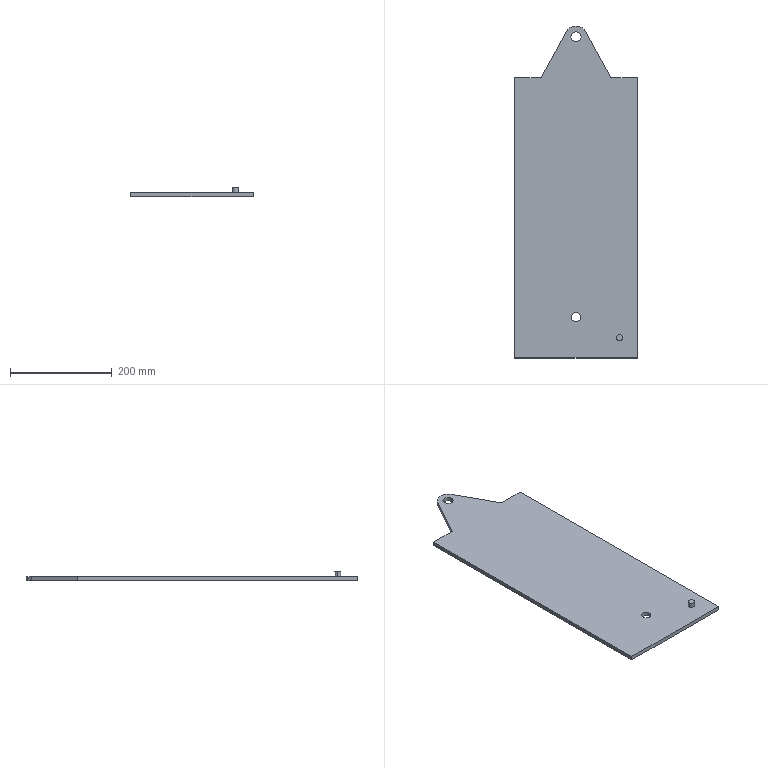Part | SolidWorks | features Extrusion 1, ICE 1 | 1 solid | 17 faces | box 240 x 651.329 x 18 mm | volume 1117831 mm3 | plane 10 | cylinder 7 | commonest cylinder face diameters 12 x2 18 x2 20 x2 42.659 x1
STEP:
#1=CARTESIAN_POINT('',(91.,40.,18.));
#2=VERTEX_POINT('',#1);
#3=CARTESIAN_POINT('',(79.,40.,18.));
#4=VERTEX_POINT('',#3);
#5=CARTESIAN_POINT('',(85.,40.,18.));
#6=DIRECTION('',(0.,0.,1.));
#7=DIRECTION('',(1.,0.,0.));
#8=AXIS2_PLACEMENT_3D('',#5,#6,#7);
#9=CIRCLE('',#8,6.);
#10=EDGE_CURVE('',#2,#4,#9,.T.);
#11=ORIENTED_EDGE('',*,*,#10,.F.);
#12=CARTESIAN_POINT('',(91.,40.,8.));
#13=VERTEX_POINT('',#12);
#14=CARTESIAN_POINT('',(91.,40.,18.));
#15=DIRECTION('',(0.,0.,-1.));
#16=VECTOR('',#15,1000.);
#17=LINE('',#14,#16);
#18=EDGE_CURVE('',#2,#13,#17,.T.);
#19=ORIENTED_EDGE('',*,*,#18,.T.);
#20=CARTESIAN_POINT('',(79.,40.,8.));
#21=VERTEX_POINT('',#20);
#22=CARTESIAN_POINT('',(85.,40.,8.));
#23=DIRECTION('',(0.,0.,1.));
#24=DIRECTION('',(1.,0.,0.));
#25=AXIS2_PLACEMENT_3D('',#22,#23,#24);
#26=CIRCLE('',#25,6.);
#27=EDGE_CURVE('',#13,#21,#26,.T.);
#28=ORIENTED_EDGE('',*,*,#27,.T.);
#29=CARTESIAN_POINT('',(79.,40.,18.));
#30=DIRECTION('',(0.,0.,-1.));
#31=VECTOR('',#30,1000.);
#32=LINE('',#29,#31);
#33=EDGE_CURVE('',#4,#21,#32,.T.);
#34=ORIENTED_EDGE('',*,*,#33,.F.);
#35=EDGE_LOOP('',(#11,#19,#28,#34));
#36=FACE_OUTER_BOUND('',#35,.T.);
#37=CARTESIAN_POINT('',(85.,40.,18.));
#38=DIRECTION('',(0.,0.,-1.));
#39=DIRECTION('',(-1.,0.,0.));
#40=AXIS2_PLACEMENT_3D('',#37,#38,#39);
#41=CYLINDRICAL_SURFACE('',#40,6.);
#42=ADVANCED_FACE('',(#36),#41,.T.);
#43=CARTESIAN_POINT('',(-9.,80.,8.));
#44=VERTEX_POINT('',#43);
#45=CARTESIAN_POINT('',(9.,80.,8.));
#46=VERTEX_POINT('',#45);
#47=CARTESIAN_POINT('',(0.,80.,8.));
#48=DIRECTION('',(0.,0.,1.));
#49=DIRECTION('',(1.,0.,0.));
#50=AXIS2_PLACEMENT_3D('',#47,#48,#49);
#51=CIRCLE('',#50,9.);
#52=EDGE_CURVE('',#44,#46,#51,.T.);
#53=ORIENTED_EDGE('',*,*,#52,.T.);
#54=CARTESIAN_POINT('',(9.,80.,0.));
#55=VERTEX_POINT('',#54);
#56=CARTESIAN_POINT('',(9.,80.,8.));
#57=DIRECTION('',(0.,0.,-1.));
#58=VECTOR('',#57,1000.);
#59=LINE('',#56,#58);
#60=EDGE_CURVE('',#46,#55,#59,.T.);
#61=ORIENTED_EDGE('',*,*,#60,.T.);
#62=CARTESIAN_POINT('',(-9.,80.,0.));
#63=VERTEX_POINT('',#62);
#64=CARTESIAN_POINT('',(0.,80.,0.));
#65=DIRECTION('',(0.,0.,1.));
#66=DIRECTION('',(1.,0.,0.));
#67=AXIS2_PLACEMENT_3D('',#64,#65,#66);
#68=CIRCLE('',#67,9.);
#69=EDGE_CURVE('',#63,#55,#68,.T.);
#70=ORIENTED_EDGE('',*,*,#69,.F.);
#71=CARTESIAN_POINT('',(-9.,80.,8.));
#72=DIRECTION('',(0.,0.,-1.));
#73=VECTOR('',#72,1000.);
#74=LINE('',#71,#73);
#75=EDGE_CURVE('',#44,#63,#74,.T.);
#76=ORIENTED_EDGE('',*,*,#75,.F.);
#77=EDGE_LOOP('',(#53,#61,#70,#76));
#78=FACE_OUTER_BOUND('',#77,.T.);
#79=CARTESIAN_POINT('',(0.,80.,8.));
#80=DIRECTION('',(0.,0.,-1.));
#81=DIRECTION('',(-1.,0.,0.));
#82=AXIS2_PLACEMENT_3D('',#79,#80,#81);
#83=CYLINDRICAL_SURFACE('',#82,9.);
#84=ADVANCED_FACE('',(#78),#83,.F.);
#85=CARTESIAN_POINT('',(-10.,630.,8.));
#86=VERTEX_POINT('',#85);
#87=CARTESIAN_POINT('',(10.,630.,8.));
#88=VERTEX_POINT('',#87);
#89=CARTESIAN_POINT('',(0.,630.,8.));
#90=DIRECTION('',(0.,0.,1.));
#91=DIRECTION('',(1.,0.,0.));
#92=AXIS2_PLACEMENT_3D('',#89,#90,#91);
#93=CIRCLE('',#92,10.);
#94=EDGE_CURVE('',#86,#88,#93,.T.);
#95=ORIENTED_EDGE('',*,*,#94,.T.);
#96=CARTESIAN_POINT('',(10.,630.,0.));
#97=VERTEX_POINT('',#96);
#98=CARTESIAN_POINT('',(10.,630.,8.));
#99=DIRECTION('',(0.,0.,-1.));
#100=VECTOR('',#99,1000.);
#101=LINE('',#98,#100);
#102=EDGE_CURVE('',#88,#97,#101,.T.);
#103=ORIENTED_EDGE('',*,*,#102,.T.);
#104=CARTESIAN_POINT('',(-10.,630.,0.));
#105=VERTEX_POINT('',#104);
#106=CARTESIAN_POINT('',(0.,630.,0.));
#107=DIRECTION('',(0.,0.,1.));
#108=DIRECTION('',(1.,0.,0.));
#109=AXIS2_PLACEMENT_3D('',#106,#107,#108);
#110=CIRCLE('',#109,10.);
#111=EDGE_CURVE('',#105,#97,#110,.T.);
#112=ORIENTED_EDGE('',*,*,#111,.F.);
#113=CARTESIAN_POINT('',(-10.,630.,8.));
#114=DIRECTION('',(0.,0.,-1.));
#115=VECTOR('',#114,1000.);
#116=LINE('',#113,#115);
#117=EDGE_CURVE('',#86,#105,#116,.T.);
#118=ORIENTED_EDGE('',*,*,#117,.F.);
#119=EDGE_LOOP('',(#95,#103,#112,#118));
#120=FACE_OUTER_BOUND('',#119,.T.);
#121=CARTESIAN_POINT('',(0.,630.,8.));
#122=DIRECTION('',(0.,0.,-1.));
#123=DIRECTION('',(-1.,0.,0.));
#124=AXIS2_PLACEMENT_3D('',#121,#122,#123);
#125=CYLINDRICAL_SURFACE('',#124,10.);
#126=ADVANCED_FACE('',(#120),#125,.F.);
#127=CARTESIAN_POINT('',(85.,40.,8.));
#128=DIRECTION('',(0.,0.,1.));
#129=DIRECTION('',(1.,0.,0.));
#130=AXIS2_PLACEMENT_3D('',#127,#128,#129);
#131=CIRCLE('',#130,6.);
#132=EDGE_CURVE('',#21,#13,#131,.T.);
#133=ORIENTED_EDGE('',*,*,#132,.F.);
#134=ORIENTED_EDGE('',*,*,#27,.F.);
#135=EDGE_LOOP('',(#133,#134));
#136=FACE_BOUND('',#135,.T.);
#137=ORIENTED_EDGE('',*,*,#94,.F.);
#138=CARTESIAN_POINT('',(0.,630.,8.));
#139=DIRECTION('',(0.,0.,1.));
#140=DIRECTION('',(1.,0.,0.));
#141=AXIS2_PLACEMENT_3D('',#138,#139,#140);
#142=CIRCLE('',#141,10.);
#143=EDGE_CURVE('',#88,#86,#142,.T.);
#144=ORIENTED_EDGE('',*,*,#143,.F.);
#145=EDGE_LOOP('',(#137,#144));
#146=FACE_BOUND('',#145,.T.);
#147=CARTESIAN_POINT('',(-120.,550.,8.));
#148=VERTEX_POINT('',#147);
#149=CARTESIAN_POINT('',(-120.,0.,8.));
#150=VERTEX_POINT('',#149);
#151=CARTESIAN_POINT('',(-120.,0.,8.));
#152=DIRECTION('',(0.,-1.,0.));
#153=VECTOR('',#152,1000.);
#154=LINE('',#151,#153);
#155=EDGE_CURVE('',#148,#150,#154,.T.);
#156=ORIENTED_EDGE('',*,*,#155,.T.);
#157=CARTESIAN_POINT('',(120.,0.,8.));
#158=VERTEX_POINT('',#157);
#159=CARTESIAN_POINT('',(120.,0.,8.));
#160=DIRECTION('',(1.,0.,0.));
#161=VECTOR('',#160,1000.);
#162=LINE('',#159,#161);
#163=EDGE_CURVE('',#150,#158,#162,.T.);
#164=ORIENTED_EDGE('',*,*,#163,.T.);
#165=CARTESIAN_POINT('',(120.,550.,8.));
#166=VERTEX_POINT('',#165);
#167=CARTESIAN_POINT('',(120.,550.,8.));
#168=DIRECTION('',(0.,1.,0.));
#169=VECTOR('',#168,1000.);
#170=LINE('',#167,#169);
#171=EDGE_CURVE('',#158,#166,#170,.T.);
#172=ORIENTED_EDGE('',*,*,#171,.T.);
#173=CARTESIAN_POINT('',(68.4,550.,8.));
#174=VERTEX_POINT('',#173);
#175=CARTESIAN_POINT('',(68.4,550.,8.));
#176=DIRECTION('',(-1.,0.,0.));
#177=VECTOR('',#176,1000.);
#178=LINE('',#175,#177);
#179=EDGE_CURVE('',#166,#174,#178,.T.);
#180=ORIENTED_EDGE('',*,*,#179,.T.);
#181=CARTESIAN_POINT('',(18.684,640.288,8.));
#182=VERTEX_POINT('',#181);
#183=CARTESIAN_POINT('',(18.684,640.288,8.));
#184=DIRECTION('',(-0.4823,0.876,0.));
#185=VECTOR('',#184,1000.);
#186=LINE('',#183,#185);
#187=EDGE_CURVE('',#174,#182,#186,.T.);
#188=ORIENTED_EDGE('',*,*,#187,.T.);
#189=CARTESIAN_POINT('',(-18.684,640.288,8.));
#190=VERTEX_POINT('',#189);
#191=CARTESIAN_POINT('',(0.,630.,8.));
#192=DIRECTION('',(0.,0.,1.));
#193=DIRECTION('',(1.,0.,0.));
#194=AXIS2_PLACEMENT_3D('',#191,#192,#193);
#195=CIRCLE('',#194,21.329);
#196=EDGE_CURVE('',#182,#190,#195,.T.);
#197=ORIENTED_EDGE('',*,*,#196,.T.);
#198=CARTESIAN_POINT('',(-68.4,550.,8.));
#199=VERTEX_POINT('',#198);
#200=CARTESIAN_POINT('',(-18.684,640.288,8.));
#201=DIRECTION('',(-0.4823,-0.876,0.));
#202=VECTOR('',#201,1000.);
#203=LINE('',#200,#202);
#204=EDGE_CURVE('',#190,#199,#203,.T.);
#205=ORIENTED_EDGE('',*,*,#204,.T.);
#206=CARTESIAN_POINT('',(-120.,550.,8.));
#207=DIRECTION('',(-1.,0.,0.));
#208=VECTOR('',#207,1000.);
#209=LINE('',#206,#208);
#210=EDGE_CURVE('',#199,#148,#209,.T.);
#211=ORIENTED_EDGE('',*,*,#210,.T.);
#212=EDGE_LOOP('',(#156,#164,#172,#180,#188,#197,#205,#211));
#213=FACE_OUTER_BOUND('',#212,.T.);
#214=ORIENTED_EDGE('',*,*,#52,.F.);
#215=CARTESIAN_POINT('',(0.,80.,8.));
#216=DIRECTION('',(0.,0.,1.));
#217=DIRECTION('',(1.,0.,0.));
#218=AXIS2_PLACEMENT_3D('',#215,#216,#217);
#219=CIRCLE('',#218,9.);
#220=EDGE_CURVE('',#46,#44,#219,.T.);
#221=ORIENTED_EDGE('',*,*,#220,.F.);
#222=EDGE_LOOP('',(#214,#221));
#223=FACE_BOUND('',#222,.T.);
#224=CARTESIAN_POINT('',(0.,630.,8.));
#225=DIRECTION('',(0.,0.,1.));
#226=DIRECTION('',(1.,0.,0.));
#227=AXIS2_PLACEMENT_3D('',#224,#225,#226);
#228=PLANE('',#227);
#229=ADVANCED_FACE('',(#136,#146,#213,#223),#228,.T.);
#230=CARTESIAN_POINT('',(-120.,550.,0.));
#231=VERTEX_POINT('',#230);
#232=CARTESIAN_POINT('',(-120.,0.,0.));
#233=VERTEX_POINT('',#232);
#234=CARTESIAN_POINT('',(-120.,0.,0.));
#235=DIRECTION('',(0.,-1.,0.));
#236=VECTOR('',#235,1000.);
#237=LINE('',#234,#236);
#238=EDGE_CURVE('',#231,#233,#237,.T.);
#239=ORIENTED_EDGE('',*,*,#238,.F.);
#240=CARTESIAN_POINT('',(-68.4,550.,0.));
#241=VERTEX_POINT('',#240);
#242=CARTESIAN_POINT('',(-120.,550.,0.));
#243=DIRECTION('',(-1.,0.,0.));
#244=VECTOR('',#243,1000.);
#245=LINE('',#242,#244);
#246=EDGE_CURVE('',#241,#231,#245,.T.);
#247=ORIENTED_EDGE('',*,*,#246,.F.);
#248=CARTESIAN_POINT('',(-18.684,640.288,0.));
#249=VERTEX_POINT('',#248);
#250=CARTESIAN_POINT('',(-18.684,640.288,0.));
#251=DIRECTION('',(-0.4823,-0.876,0.));
#252=VECTOR('',#251,1000.);
#253=LINE('',#250,#252);
#254=EDGE_CURVE('',#249,#241,#253,.T.);
#255=ORIENTED_EDGE('',*,*,#254,.F.);
#256=CARTESIAN_POINT('',(18.684,640.288,0.));
#257=VERTEX_POINT('',#256);
#258=CARTESIAN_POINT('',(0.,630.,0.));
#259=DIRECTION('',(0.,0.,1.));
#260=DIRECTION('',(1.,0.,0.));
#261=AXIS2_PLACEMENT_3D('',#258,#259,#260);
#262=CIRCLE('',#261,21.329);
#263=EDGE_CURVE('',#257,#249,#262,.T.);
#264=ORIENTED_EDGE('',*,*,#263,.F.);
#265=CARTESIAN_POINT('',(68.4,550.,0.));
#266=VERTEX_POINT('',#265);
#267=CARTESIAN_POINT('',(18.684,640.288,0.));
#268=DIRECTION('',(-0.4823,0.876,0.));
#269=VECTOR('',#268,1000.);
#270=LINE('',#267,#269);
#271=EDGE_CURVE('',#266,#257,#270,.T.);
#272=ORIENTED_EDGE('',*,*,#271,.F.);
#273=CARTESIAN_POINT('',(120.,550.,0.));
#274=VERTEX_POINT('',#273);
#275=CARTESIAN_POINT('',(68.4,550.,0.));
#276=DIRECTION('',(-1.,0.,0.));
#277=VECTOR('',#276,1000.);
#278=LINE('',#275,#277);
#279=EDGE_CURVE('',#274,#266,#278,.T.);
#280=ORIENTED_EDGE('',*,*,#279,.F.);
#281=CARTESIAN_POINT('',(120.,0.,0.));
#282=VERTEX_POINT('',#281);
#283=CARTESIAN_POINT('',(120.,550.,0.));
#284=DIRECTION('',(0.,1.,0.));
#285=VECTOR('',#284,1000.);
#286=LINE('',#283,#285);
#287=EDGE_CURVE('',#282,#274,#286,.T.);
#288=ORIENTED_EDGE('',*,*,#287,.F.);
#289=CARTESIAN_POINT('',(120.,0.,0.));
#290=DIRECTION('',(1.,0.,0.));
#291=VECTOR('',#290,1000.);
#292=LINE('',#289,#291);
#293=EDGE_CURVE('',#233,#282,#292,.T.);
#294=ORIENTED_EDGE('',*,*,#293,.F.);
#295=EDGE_LOOP('',(#239,#247,#255,#264,#272,#280,#288,#294));
#296=FACE_OUTER_BOUND('',#295,.T.);
#297=ORIENTED_EDGE('',*,*,#111,.T.);
#298=CARTESIAN_POINT('',(0.,630.,0.));
#299=DIRECTION('',(0.,0.,1.));
#300=DIRECTION('',(1.,0.,0.));
#301=AXIS2_PLACEMENT_3D('',#298,#299,#300);
#302=CIRCLE('',#301,10.);
#303=EDGE_CURVE('',#97,#105,#302,.T.);
#304=ORIENTED_EDGE('',*,*,#303,.T.);
#305=EDGE_LOOP('',(#297,#304));
#306=FACE_BOUND('',#305,.T.);
#307=ORIENTED_EDGE('',*,*,#69,.T.);
#308=CARTESIAN_POINT('',(0.,80.,0.));
#309=DIRECTION('',(0.,0.,1.));
#310=DIRECTION('',(1.,0.,0.));
#311=AXIS2_PLACEMENT_3D('',#308,#309,#310);
#312=CIRCLE('',#311,9.);
#313=EDGE_CURVE('',#55,#63,#312,.T.);
#314=ORIENTED_EDGE('',*,*,#313,.T.);
#315=EDGE_LOOP('',(#307,#314));
#316=FACE_BOUND('',#315,.T.);
#317=CARTESIAN_POINT('',(0.,630.,0.));
#318=DIRECTION('',(0.,0.,1.));
#319=DIRECTION('',(1.,0.,0.));
#320=AXIS2_PLACEMENT_3D('',#317,#318,#319);
#321=PLANE('',#320);
#322=ADVANCED_FACE('',(#296,#306,#316),#321,.F.);
#323=ORIENTED_EDGE('',*,*,#238,.T.);
#324=CARTESIAN_POINT('',(-120.,0.,8.));
#325=DIRECTION('',(0.,0.,-1.));
#326=VECTOR('',#325,1000.);
#327=LINE('',#324,#326);
#328=EDGE_CURVE('',#150,#233,#327,.T.);
#329=ORIENTED_EDGE('',*,*,#328,.F.);
#330=ORIENTED_EDGE('',*,*,#155,.F.);
#331=CARTESIAN_POINT('',(-120.,550.,8.));
#332=DIRECTION('',(0.,0.,-1.));
#333=VECTOR('',#332,1000.);
#334=LINE('',#331,#333);
#335=EDGE_CURVE('',#148,#231,#334,.T.);
#336=ORIENTED_EDGE('',*,*,#335,.T.);
#337=EDGE_LOOP('',(#323,#329,#330,#336));
#338=FACE_OUTER_BOUND('',#337,.T.);
#339=CARTESIAN_POINT('',(-120.,0.,8.));
#340=DIRECTION('',(1.,0.,0.));
#341=DIRECTION('',(0.,1.,0.));
#342=AXIS2_PLACEMENT_3D('',#339,#340,#341);
#343=PLANE('',#342);
#344=ADVANCED_FACE('',(#338),#343,.F.);
#345=ORIENTED_EDGE('',*,*,#293,.T.);
#346=CARTESIAN_POINT('',(120.,0.,8.));
#347=DIRECTION('',(0.,0.,-1.));
#348=VECTOR('',#347,1000.);
#349=LINE('',#346,#348);
#350=EDGE_CURVE('',#158,#282,#349,.T.);
#351=ORIENTED_EDGE('',*,*,#350,.F.);
#352=ORIENTED_EDGE('',*,*,#163,.F.);
#353=ORIENTED_EDGE('',*,*,#328,.T.);
#354=EDGE_LOOP('',(#345,#351,#352,#353));
#355=FACE_OUTER_BOUND('',#354,.T.);
#356=CARTESIAN_POINT('',(120.,0.,8.));
#357=DIRECTION('',(0.,1.,0.));
#358=DIRECTION('',(-1.,0.,0.));
#359=AXIS2_PLACEMENT_3D('',#356,#357,#358);
#360=PLANE('',#359);
#361=ADVANCED_FACE('',(#355),#360,.F.);
#362=ORIENTED_EDGE('',*,*,#287,.T.);
#363=CARTESIAN_POINT('',(120.,550.,8.));
#364=DIRECTION('',(0.,0.,-1.));
#365=VECTOR('',#364,1000.);
#366=LINE('',#363,#365);
#367=EDGE_CURVE('',#166,#274,#366,.T.);
#368=ORIENTED_EDGE('',*,*,#367,.F.);
#369=ORIENTED_EDGE('',*,*,#171,.F.);
#370=ORIENTED_EDGE('',*,*,#350,.T.);
#371=EDGE_LOOP('',(#362,#368,#369,#370));
#372=FACE_OUTER_BOUND('',#371,.T.);
#373=CARTESIAN_POINT('',(120.,550.,8.));
#374=DIRECTION('',(-1.,0.,0.));
#375=DIRECTION('',(0.,-1.,0.));
#376=AXIS2_PLACEMENT_3D('',#373,#374,#375);
#377=PLANE('',#376);
#378=ADVANCED_FACE('',(#372),#377,.F.);
#379=ORIENTED_EDGE('',*,*,#279,.T.);
#380=CARTESIAN_POINT('',(68.4,550.,8.));
#381=DIRECTION('',(0.,0.,-1.));
#382=VECTOR('',#381,1000.);
#383=LINE('',#380,#382);
#384=EDGE_CURVE('',#174,#266,#383,.T.);
#385=ORIENTED_EDGE('',*,*,#384,.F.);
#386=ORIENTED_EDGE('',*,*,#179,.F.);
#387=ORIENTED_EDGE('',*,*,#367,.T.);
#388=EDGE_LOOP('',(#379,#385,#386,#387));
#389=FACE_OUTER_BOUND('',#388,.T.);
#390=CARTESIAN_POINT('',(68.4,550.,8.));
#391=DIRECTION('',(0.,-1.,0.));
#392=DIRECTION('',(0.,0.,-1.));
#393=AXIS2_PLACEMENT_3D('',#390,#391,#392);
#394=PLANE('',#393);
#395=ADVANCED_FACE('',(#389),#394,.F.);
#396=ORIENTED_EDGE('',*,*,#271,.T.);
#397=CARTESIAN_POINT('',(18.684,640.288,8.));
#398=DIRECTION('',(0.,0.,-1.));
#399=VECTOR('',#398,1000.);
#400=LINE('',#397,#399);
#401=EDGE_CURVE('',#182,#257,#400,.T.);
#402=ORIENTED_EDGE('',*,*,#401,.F.);
#403=ORIENTED_EDGE('',*,*,#187,.F.);
#404=ORIENTED_EDGE('',*,*,#384,.T.);
#405=EDGE_LOOP('',(#396,#402,#403,#404));
#406=FACE_OUTER_BOUND('',#405,.T.);
#407=CARTESIAN_POINT('',(18.684,640.288,8.));
#408=DIRECTION('',(-0.876,-0.4823,0.));
#409=DIRECTION('',(0.4823,-0.876,0.));
#410=AXIS2_PLACEMENT_3D('',#407,#408,#409);
#411=PLANE('',#410);
#412=ADVANCED_FACE('',(#406),#411,.F.);
#413=ORIENTED_EDGE('',*,*,#263,.T.);
#414=CARTESIAN_POINT('',(-18.684,640.288,8.));
#415=DIRECTION('',(0.,0.,-1.));
#416=VECTOR('',#415,1000.);
#417=LINE('',#414,#416);
#418=EDGE_CURVE('',#190,#249,#417,.T.);
#419=ORIENTED_EDGE('',*,*,#418,.F.);
#420=ORIENTED_EDGE('',*,*,#196,.F.);
#421=ORIENTED_EDGE('',*,*,#401,.T.);
#422=EDGE_LOOP('',(#413,#419,#420,#421));
#423=FACE_OUTER_BOUND('',#422,.T.);
#424=CARTESIAN_POINT('',(0.,630.,8.));
#425=DIRECTION('',(0.,0.,-1.));
#426=DIRECTION('',(-1.,0.,0.));
#427=AXIS2_PLACEMENT_3D('',#424,#425,#426);
#428=CYLINDRICAL_SURFACE('',#427,21.329);
#429=ADVANCED_FACE('',(#423),#428,.T.);
#430=ORIENTED_EDGE('',*,*,#254,.T.);
#431=CARTESIAN_POINT('',(-68.4,550.,8.));
#432=DIRECTION('',(0.,0.,-1.));
#433=VECTOR('',#432,1000.);
#434=LINE('',#431,#433);
#435=EDGE_CURVE('',#199,#241,#434,.T.);
#436=ORIENTED_EDGE('',*,*,#435,.F.);
#437=ORIENTED_EDGE('',*,*,#204,.F.);
#438=ORIENTED_EDGE('',*,*,#418,.T.);
#439=EDGE_LOOP('',(#430,#436,#437,#438));
#440=FACE_OUTER_BOUND('',#439,.T.);
#441=CARTESIAN_POINT('',(-18.684,640.288,8.));
#442=DIRECTION('',(0.876,-0.4823,0.));
#443=DIRECTION('',(0.4823,0.876,0.));
#444=AXIS2_PLACEMENT_3D('',#441,#442,#443);
#445=PLANE('',#444);
#446=ADVANCED_FACE('',(#440),#445,.F.);
#447=ORIENTED_EDGE('',*,*,#246,.T.);
#448=ORIENTED_EDGE('',*,*,#335,.F.);
#449=ORIENTED_EDGE('',*,*,#210,.F.);
#450=ORIENTED_EDGE('',*,*,#435,.T.);
#451=EDGE_LOOP('',(#447,#448,#449,#450));
#452=FACE_OUTER_BOUND('',#451,.T.);
#453=CARTESIAN_POINT('',(-120.,550.,8.));
#454=DIRECTION('',(0.,-1.,0.));
#455=DIRECTION('',(0.,0.,-1.));
#456=AXIS2_PLACEMENT_3D('',#453,#454,#455);
#457=PLANE('',#456);
#458=ADVANCED_FACE('',(#452),#457,.F.);
#459=ORIENTED_EDGE('',*,*,#102,.F.);
#460=ORIENTED_EDGE('',*,*,#143,.T.);
#461=ORIENTED_EDGE('',*,*,#117,.T.);
#462=ORIENTED_EDGE('',*,*,#303,.F.);
#463=EDGE_LOOP('',(#459,#460,#461,#462));
#464=FACE_OUTER_BOUND('',#463,.T.);
#465=CARTESIAN_POINT('',(0.,630.,8.));
#466=DIRECTION('',(0.,0.,-1.));
#467=DIRECTION('',(-1.,0.,0.));
#468=AXIS2_PLACEMENT_3D('',#465,#466,#467);
#469=CYLINDRICAL_SURFACE('',#468,10.);
#470=ADVANCED_FACE('',(#464),#469,.F.);
#471=ORIENTED_EDGE('',*,*,#60,.F.);
#472=ORIENTED_EDGE('',*,*,#220,.T.);
#473=ORIENTED_EDGE('',*,*,#75,.T.);
#474=ORIENTED_EDGE('',*,*,#313,.F.);
#475=EDGE_LOOP('',(#471,#472,#473,#474));
#476=FACE_OUTER_BOUND('',#475,.T.);
#477=CARTESIAN_POINT('',(0.,80.,8.));
#478=DIRECTION('',(0.,0.,-1.));
#479=DIRECTION('',(-1.,0.,0.));
#480=AXIS2_PLACEMENT_3D('',#477,#478,#479);
#481=CYLINDRICAL_SURFACE('',#480,9.);
#482=ADVANCED_FACE('',(#476),#481,.F.);
#483=ORIENTED_EDGE('',*,*,#18,.F.);
#484=CARTESIAN_POINT('',(85.,40.,18.));
#485=DIRECTION('',(0.,0.,1.));
#486=DIRECTION('',(1.,0.,0.));
#487=AXIS2_PLACEMENT_3D('',#484,#485,#486);
#488=CIRCLE('',#487,6.);
#489=EDGE_CURVE('',#4,#2,#488,.T.);
#490=ORIENTED_EDGE('',*,*,#489,.F.);
#491=ORIENTED_EDGE('',*,*,#33,.T.);
#492=ORIENTED_EDGE('',*,*,#132,.T.);
#493=EDGE_LOOP('',(#483,#490,#491,#492));
#494=FACE_OUTER_BOUND('',#493,.T.);
#495=CARTESIAN_POINT('',(85.,40.,18.));
#496=DIRECTION('',(0.,0.,-1.));
#497=DIRECTION('',(-1.,0.,0.));
#498=AXIS2_PLACEMENT_3D('',#495,#496,#497);
#499=CYLINDRICAL_SURFACE('',#498,6.);
#500=ADVANCED_FACE('',(#494),#499,.T.);
#501=ORIENTED_EDGE('',*,*,#489,.T.);
#502=ORIENTED_EDGE('',*,*,#10,.T.);
#503=EDGE_LOOP('',(#501,#502));
#504=FACE_OUTER_BOUND('',#503,.T.);
#505=CARTESIAN_POINT('',(85.,40.,18.));
#506=DIRECTION('',(0.,0.,1.));
#507=DIRECTION('',(1.,0.,0.));
#508=AXIS2_PLACEMENT_3D('',#505,#506,#507);
#509=PLANE('',#508);
#510=ADVANCED_FACE('',(#504),#509,.T.);
#511=CLOSED_SHELL('',(#42,#84,#126,#229,#322,#344,#361,#378,#395,#412,#429,#446,#458,#470,#482,#500,#510));
#512=MANIFOLD_SOLID_BREP('',#511);
#513=CARTESIAN_POINT('',(0.,0.,0.));
#514=DIRECTION('',(0.,0.,1.));
#515=DIRECTION('',(1.,0.,0.));
#516=AXIS2_PLACEMENT_3D('',#513,#514,#515);
#517=(LENGTH_UNIT()NAMED_UNIT(*)SI_UNIT(.MILLI.,.METRE.));
#518=UNCERTAINTY_MEASURE_WITH_UNIT(LENGTH_MEASURE(0.00001),#517,'','');
#519=(NAMED_UNIT(*)PLANE_ANGLE_UNIT()SI_UNIT($,.RADIAN.));
#520=(NAMED_UNIT(*)SI_UNIT($,.STERADIAN.)SOLID_ANGLE_UNIT());
#521=(GEOMETRIC_REPRESENTATION_CONTEXT(3)GLOBAL_UNCERTAINTY_ASSIGNED_CONTEXT((#518))GLOBAL_UNIT_ASSIGNED_CONTEXT((#517,#519,#520))REPRESENTATION_CONTEXT('',''));
#522=ADVANCED_BREP_SHAPE_REPRESENTATION('',(#512,#516),#521);